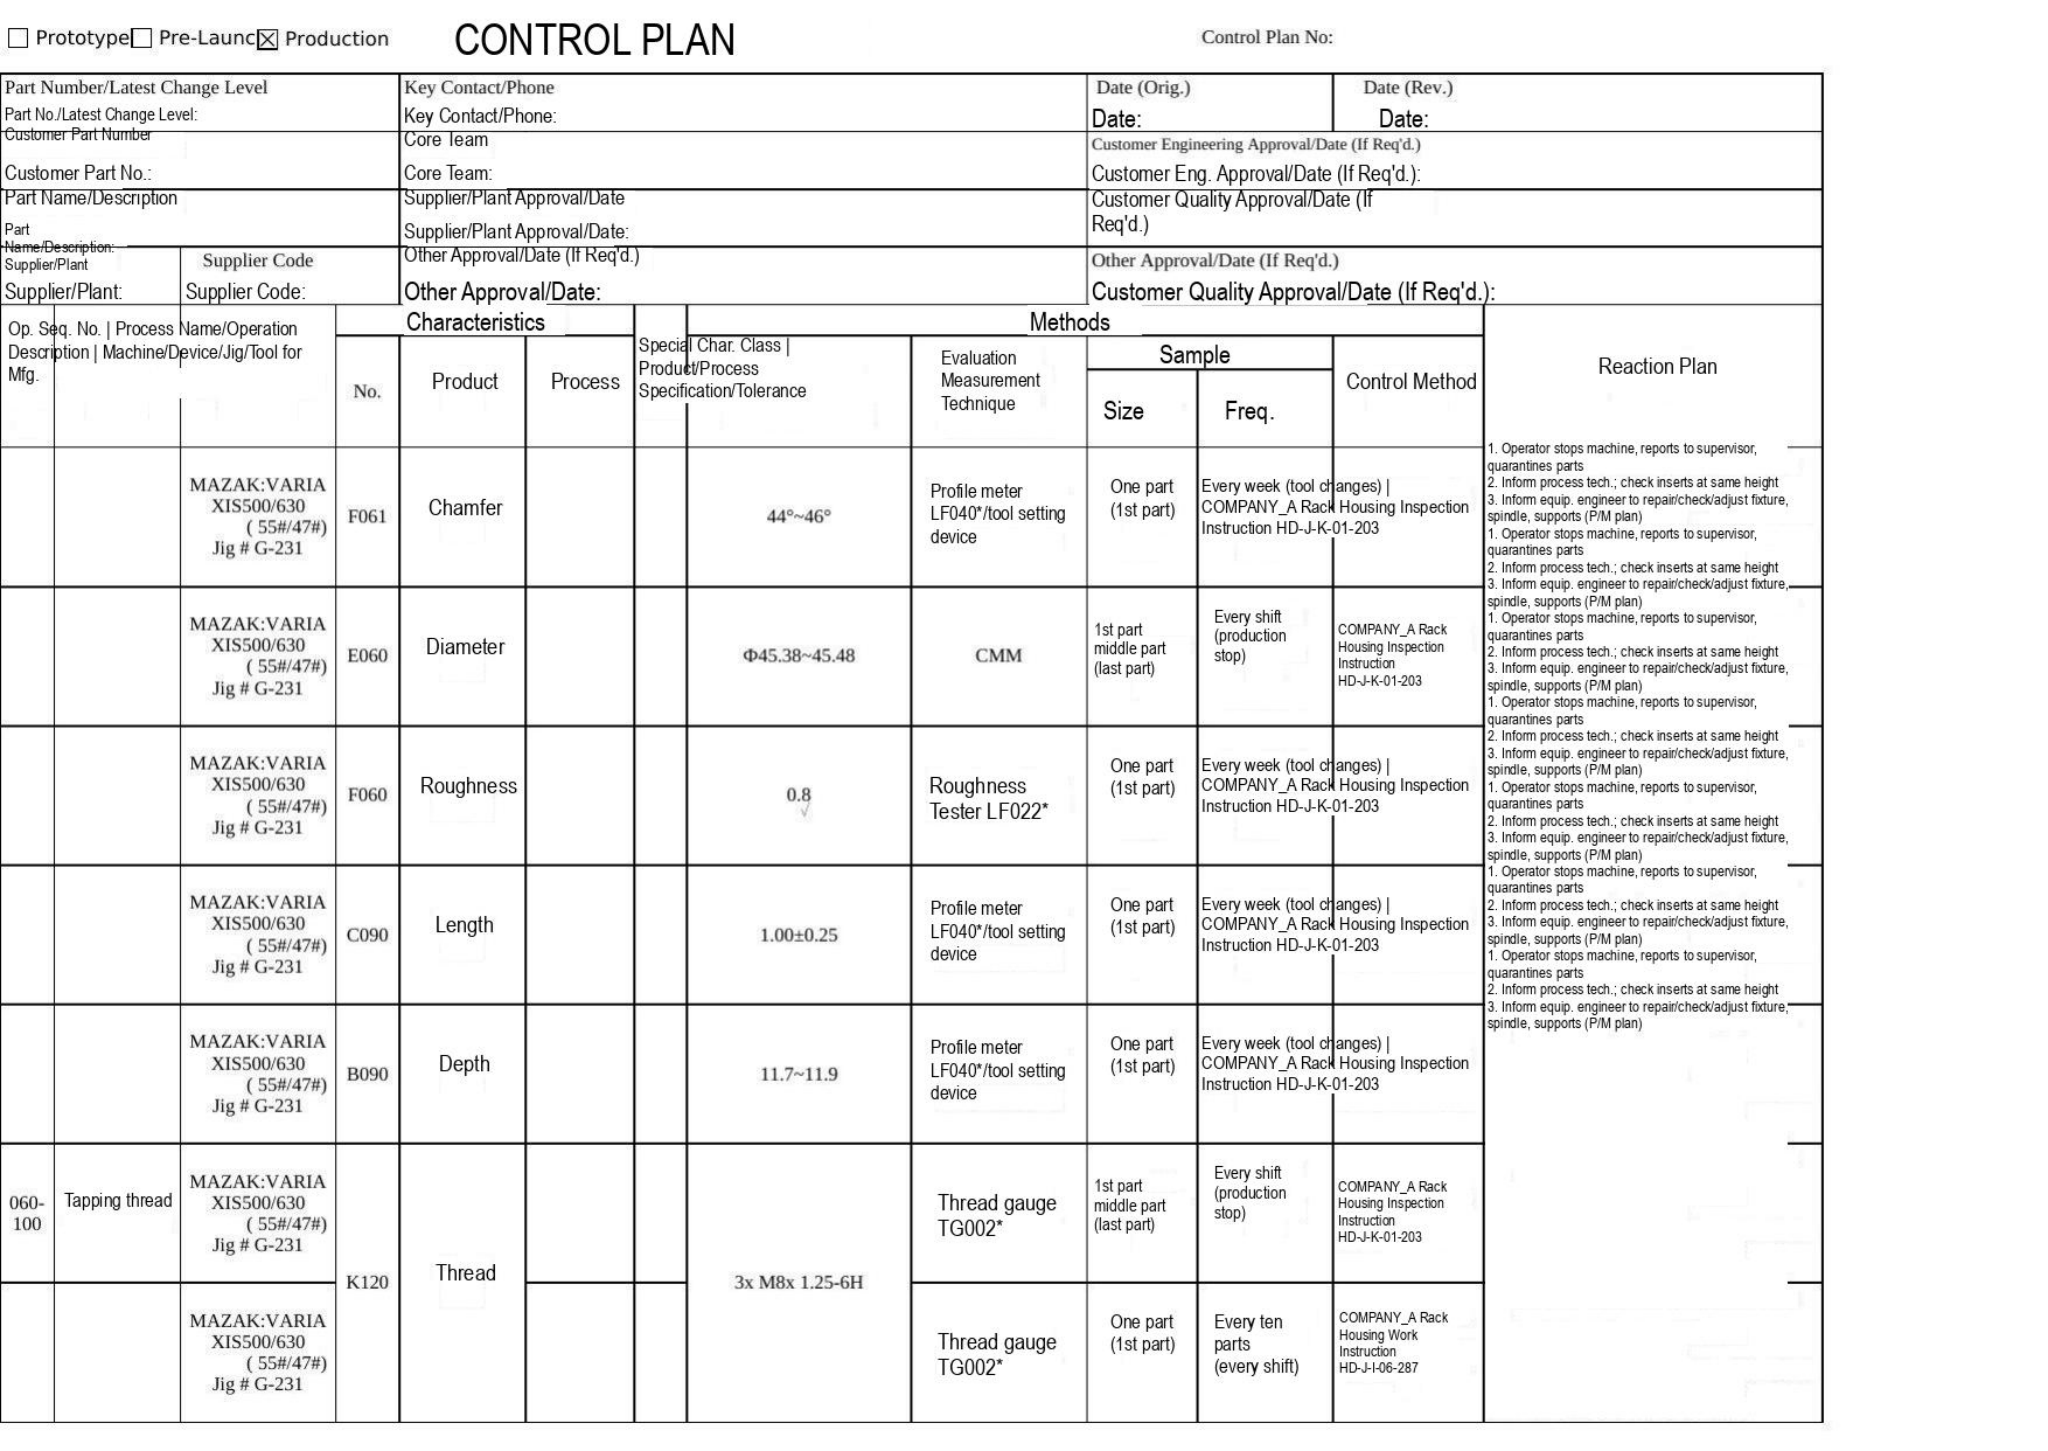☐ Prototype ☐ Pre-Launc ☒ Production

CONTROL PLAN

Control Plan No:

| Part Number/Latest Change Level<br>Part No./Latest Change Level: | | Key Contact/Phone<br>Key Contact/Phone: | Date (Orig.)<br>Date: | Date (Rev.)<br>Date: |
|---|---|---|---|---|
| Customer Part Number<br>Customer Part No.: | | Core Team<br>Core Team: | Customer Engineering Approval/Date (If Req'd.)<br>Customer Eng. Approval/Date (If Req'd.): | |
| Part Name/Description<br>Part Name/Description: | | Supplier/Plant Approval/Date<br>Supplier/Plant Approval/Date: | Customer Quality Approval/Date (If Req'd.) | |
| Supplier/Plant<br>Supplier/Plant: | Supplier Code<br>Supplier Code: | Other Approval/Date (If Req'd.)<br>Other Approval/Date: | Other Approval/Date (If Req'd.)<br>Customer Quality Approval/Date (If Req'd.): | |

| Op. Seq. No. | Process Name/Operation Description | Machine/Device/Jig/Tool for Mfg. | Characteristics<br>No. | Characteristics<br>Product | Characteristics<br>Process | Special Char. Class | Product/Process Specification/Tolerance | Methods<br>Evaluation Measurement Technique | Sample<br>Size | Sample<br>Freq. | Control Method | Reaction Plan |
|---|---|---|---|---|---|---|---|---|---|---|---|---|
| | | MAZAK:VARIA XIS500/630 ( 55#/47#) Jig # G-231 | F061 | Chamfer | | | 44°~46° | Profile meter LF040*/tool setting device | One part (1st part) | Every week (tool changes) \| | COMPANY_A Rack Housing Inspection Instruction HD-J-K-01-203 | 1. Operator stops machine, reports to supervisor, quarantines parts 2. Inform process tech.; check inserts at same height 3. Inform equip. engineer to repair/check/adjust fixture, spindle, supports (P/M plan) |
| | | MAZAK:VARIA XIS500/630 ( 55#/47#) Jig # G-231 | E060 | Diameter | | | Φ45.38~45.48 | CMM | 1st part middle part (last part) | Every shift (production stop) | COMPANY_A Rack Housing Inspection Instruction HD-J-K-01-203 | 1. Operator stops machine, reports to supervisor, quarantines parts 2. Inform process tech.; check inserts at same height 3. Inform equip. engineer to repair/check/adjust fixture, spindle, supports (P/M plan) |
| | | MAZAK:VARIA XIS500/630 ( 55#/47#) Jig # G-231 | F060 | Roughness | | | 0.8 | Roughness Tester LF022* | One part (1st part) | Every week (tool changes) \| | COMPANY_A Rack Housing Inspection Instruction HD-J-K-01-203 | 1. Operator stops machine, reports to supervisor, quarantines parts 2. Inform process tech.; check inserts at same height 3. Inform equip. engineer to repair/check/adjust fixture, spindle, supports (P/M plan) |
| | | MAZAK:VARIA XIS500/630 ( 55#/47#) Jig # G-231 | C090 | Length | | | 1.00±0.25 | Profile meter LF040*/tool setting device | One part (1st part) | Every week (tool changes) \| | COMPANY_A Rack Housing Inspection Instruction HD-J-K-01-203 | 1. Operator stops machine, reports to supervisor, quarantines parts 2. Inform process tech.; check inserts at same height 3. Inform equip. engineer to repair/check/adjust fixture, spindle, supports (P/M plan) |
| | | MAZAK:VARIA XIS500/630 ( 55#/47#) Jig # G-231 | B090 | Depth | | | 11.7~11.9 | Profile meter LF040*/tool setting device | One part (1st part) | Every week (tool changes) \| | COMPANY_A Rack Housing Inspection Instruction HD-J-K-01-203 | 1. Operator stops machine, reports to supervisor, quarantines parts 2. Inform process tech.; check inserts at same height 3. Inform equip. engineer to repair/check/adjust fixture, spindle, supports (P/M plan) |
| 060-100 | Tapping thread | MAZAK:VARIA XIS500/630 ( 55#/47#) Jig # G-231 | K120 | Thread | | | 3x M8x 1.25-6H | Thread gauge TG002* | 1st part middle part (last part) | Every shift (production stop) | COMPANY_A Rack Housing Inspection Instruction HD-J-K-01-203 | 1. Operator stops machine, reports to supervisor, quarantines parts 2. Inform process tech.; check inserts at same height 3. Inform equip. engineer to repair/check/adjust fixture, spindle, supports (P/M plan) |
| | | MAZAK:VARIA XIS500/630 ( 55#/47#) Jig # G-231 | | | | | | Thread gauge TG002* | One part (1st part) | Every ten parts (every shift) | COMPANY_A Rack Housing Work Instruction HD-J-I-06-287 | 1. Operator stops machine, reports to supervisor, quarantines parts 2. Inform process tech.; check inserts at same height 3. Inform equip. engineer to repair/check/adjust fixture, spindle, supports (P/M plan) |
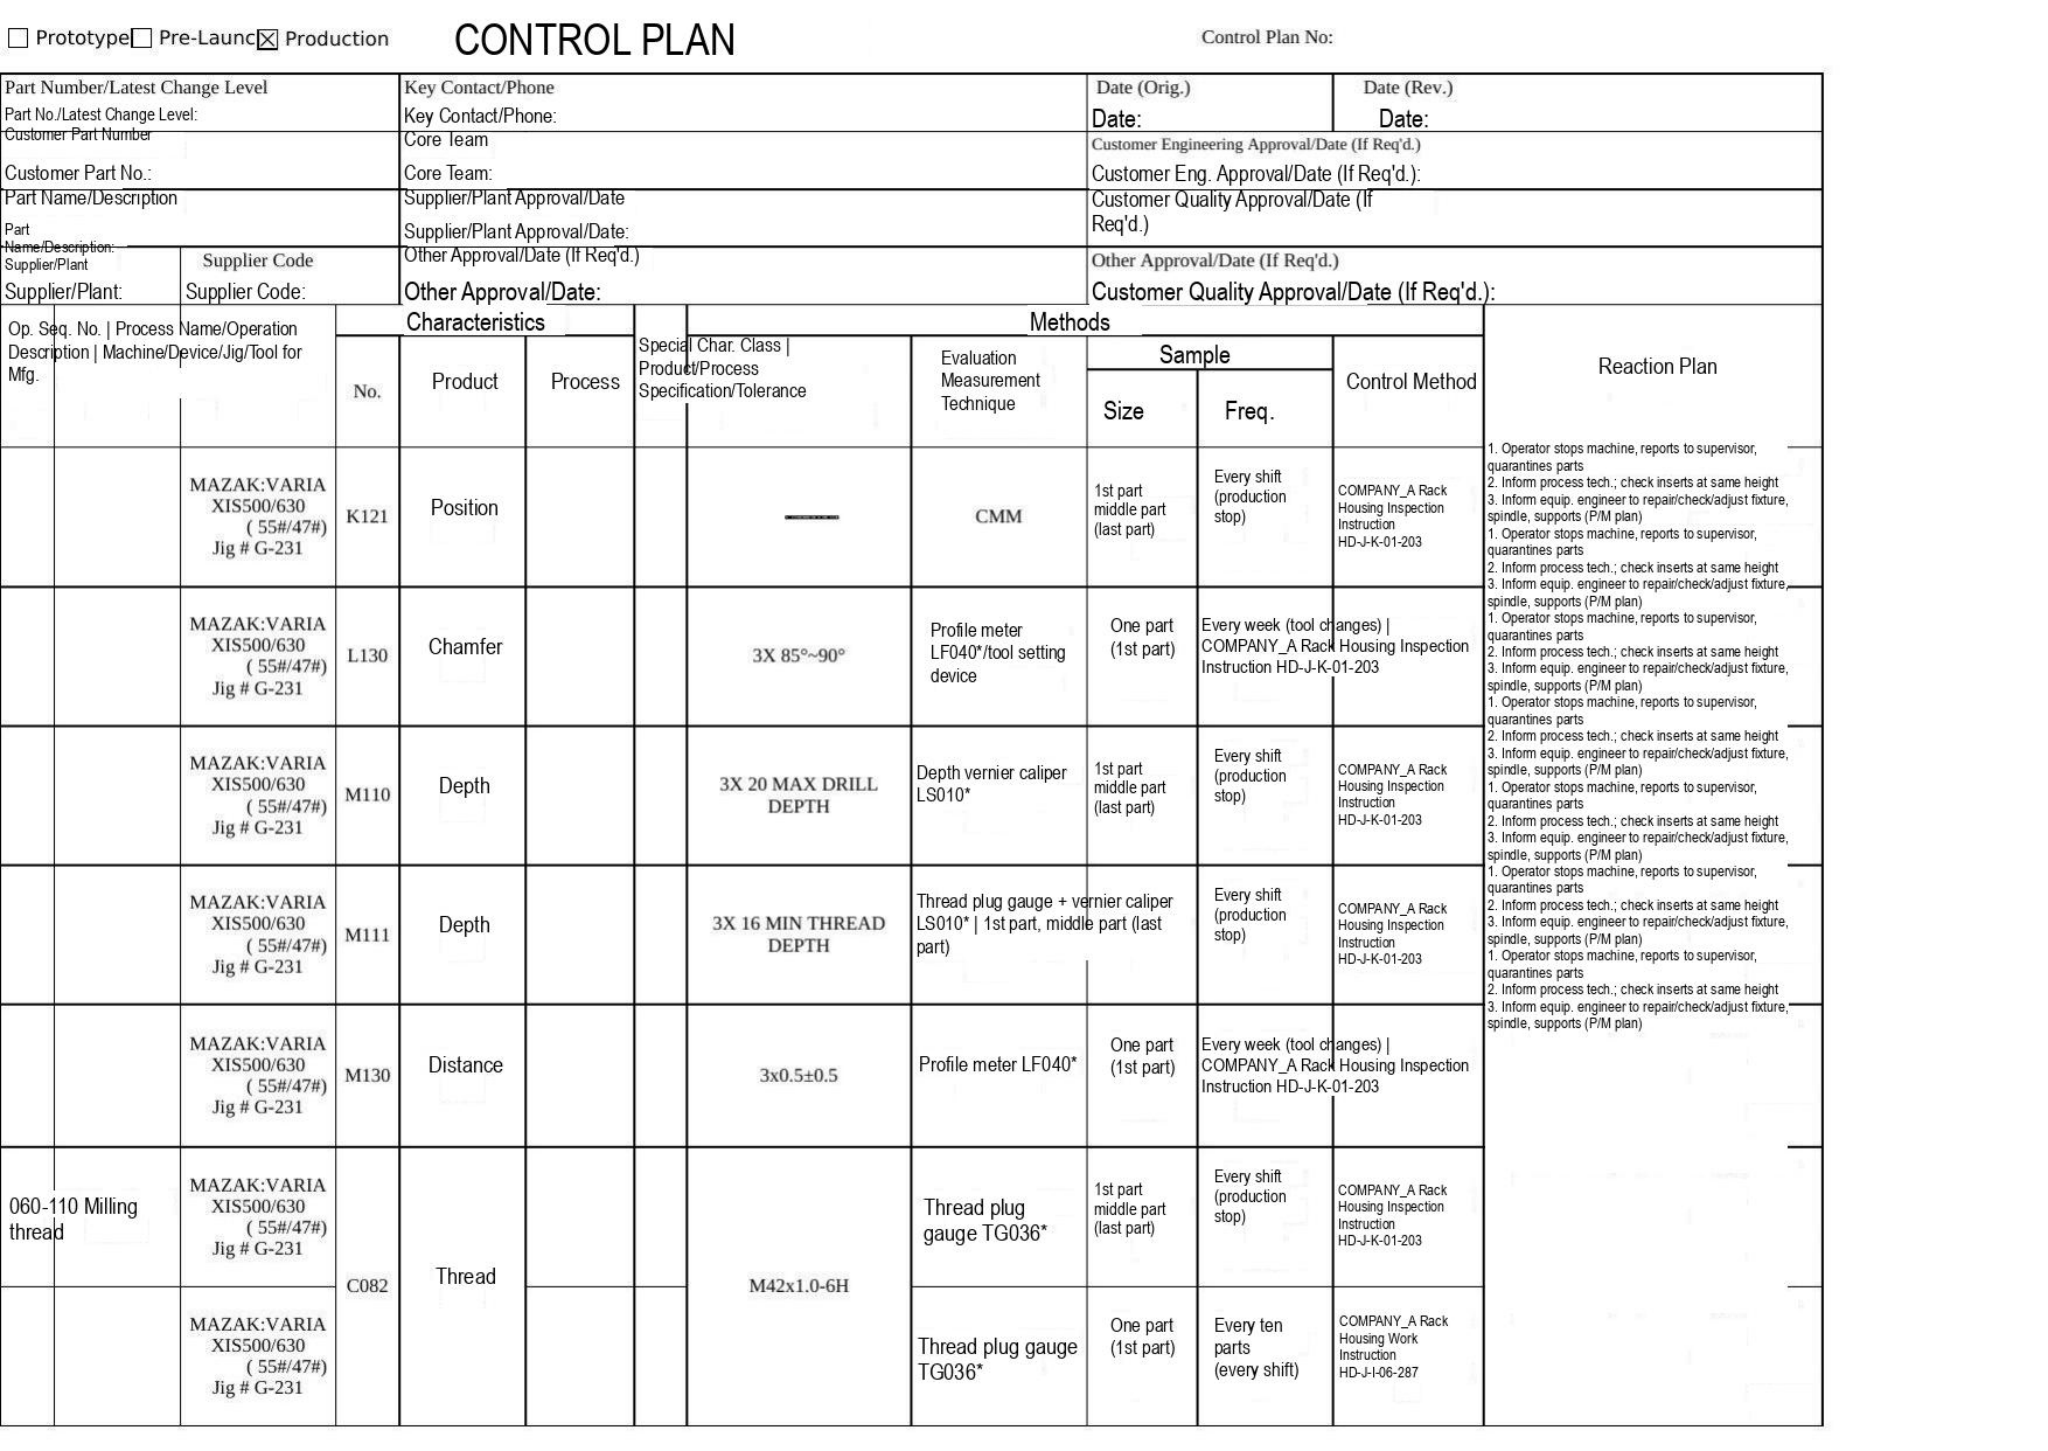☐ Prototype ☐ Pre-Launc ☒ Production

# CONTROL PLAN

Control Plan No:

| Part Number/Latest Change Level<br>Part No./Latest Change Level: | | Key Contact/Phone<br>Key Contact/Phone: | Date (Orig.)<br>Date: | Date (Rev.)<br>Date: |
|---|---|---|---|---|
| Customer Part Number<br>Customer Part No.: | | Core Team<br>Core Team: | Customer Engineering Approval/Date (If Req'd.)<br>Customer Eng. Approval/Date (If Req'd.): | |
| Part Name/Description<br>Part Name/Description: | | Supplier/Plant Approval/Date<br>Supplier/Plant Approval/Date: | Customer Quality Approval/Date (If Req'd.) | |
| Supplier/Plant<br>Supplier/Plant: | Supplier Code<br>Supplier Code: | Other Approval/Date (If Req'd.)<br>Other Approval/Date: | Other Approval/Date (If Req'd.)<br>Customer Quality Approval/Date (If Req'd.): | |

| Op. Seq. No. \| Process Name/Operation Description \| Machine/Device/Jig/Tool for Mfg. | | | Characteristics | | | | | Methods | | | | Reaction Plan |
|---|---|---|---|---|---|---|---|---|---|---|---|---|
| | | | No. | Product | Process | Special Char. Class \| Product/Process Specification/Tolerance | | Evaluation Measurement Technique | Sample Size | Sample Freq. | Control Method | |
| | | MAZAK:VARIA XIS500/630 ( 55#/47#) Jig # G-231 | K121 | Position | | | — | CMM | 1st part middle part (last part) | Every shift (production stop) | COMPANY_A Rack Housing Inspection Instruction HD-J-K-01-203 | 1. Operator stops machine, reports to supervisor, quarantines parts<br>2. Inform process tech.; check inserts at same height<br>3. Inform equip. engineer to repair/check/adjust fixture, spindle, supports (P/M plan) |
| | | MAZAK:VARIA XIS500/630 ( 55#/47#) Jig # G-231 | L130 | Chamfer | | | 3X 85°~90° | Profile meter LF040*/tool setting device | One part (1st part) | Every week (tool changes) \| COMPANY_A Rack Housing Inspection Instruction HD-J-K-01-203 | | 1. Operator stops machine, reports to supervisor, quarantines parts<br>2. Inform process tech.; check inserts at same height<br>3. Inform equip. engineer to repair/check/adjust fixture, spindle, supports (P/M plan) |
| | | MAZAK:VARIA XIS500/630 ( 55#/47#) Jig # G-231 | M110 | Depth | | | 3X 20 MAX DRILL DEPTH | Depth vernier caliper LS010* | 1st part middle part (last part) | Every shift (production stop) | COMPANY_A Rack Housing Inspection Instruction HD-J-K-01-203 | 1. Operator stops machine, reports to supervisor, quarantines parts<br>2. Inform process tech.; check inserts at same height<br>3. Inform equip. engineer to repair/check/adjust fixture, spindle, supports (P/M plan) |
| | | MAZAK:VARIA XIS500/630 ( 55#/47#) Jig # G-231 | M111 | Depth | | | 3X 16 MIN THREAD DEPTH | Thread plug gauge + vernier caliper LS010* \| 1st part, middle part (last part) | | Every shift (production stop) | COMPANY_A Rack Housing Inspection Instruction HD-J-K-01-203 | 1. Operator stops machine, reports to supervisor, quarantines parts<br>2. Inform process tech.; check inserts at same height<br>3. Inform equip. engineer to repair/check/adjust fixture, spindle, supports (P/M plan) |
| | | MAZAK:VARIA XIS500/630 ( 55#/47#) Jig # G-231 | M130 | Distance | | | 3x0.5±0.5 | Profile meter LF040* | One part (1st part) | Every week (tool changes) \| COMPANY_A Rack Housing Inspection Instruction HD-J-K-01-203 | | 1. Operator stops machine, reports to supervisor, quarantines parts<br>2. Inform process tech.; check inserts at same height<br>3. Inform equip. engineer to repair/check/adjust fixture, spindle, supports (P/M plan) |
| 060-110 Milling thread | | MAZAK:VARIA XIS500/630 ( 55#/47#) Jig # G-231 | C082 | Thread | | | M42x1.0-6H | Thread plug gauge TG036* | 1st part middle part (last part) | Every shift (production stop) | COMPANY_A Rack Housing Inspection Instruction HD-J-K-01-203 | 1. Operator stops machine, reports to supervisor, quarantines parts<br>2. Inform process tech.; check inserts at same height<br>3. Inform equip. engineer to repair/check/adjust fixture, spindle, supports (P/M plan) |
| | | MAZAK:VARIA XIS500/630 ( 55#/47#) Jig # G-231 | | | | | | Thread plug gauge TG036* | One part (1st part) | Every ten parts (every shift) | COMPANY_A Rack Housing Work Instruction HD-J-I-06-287 | |
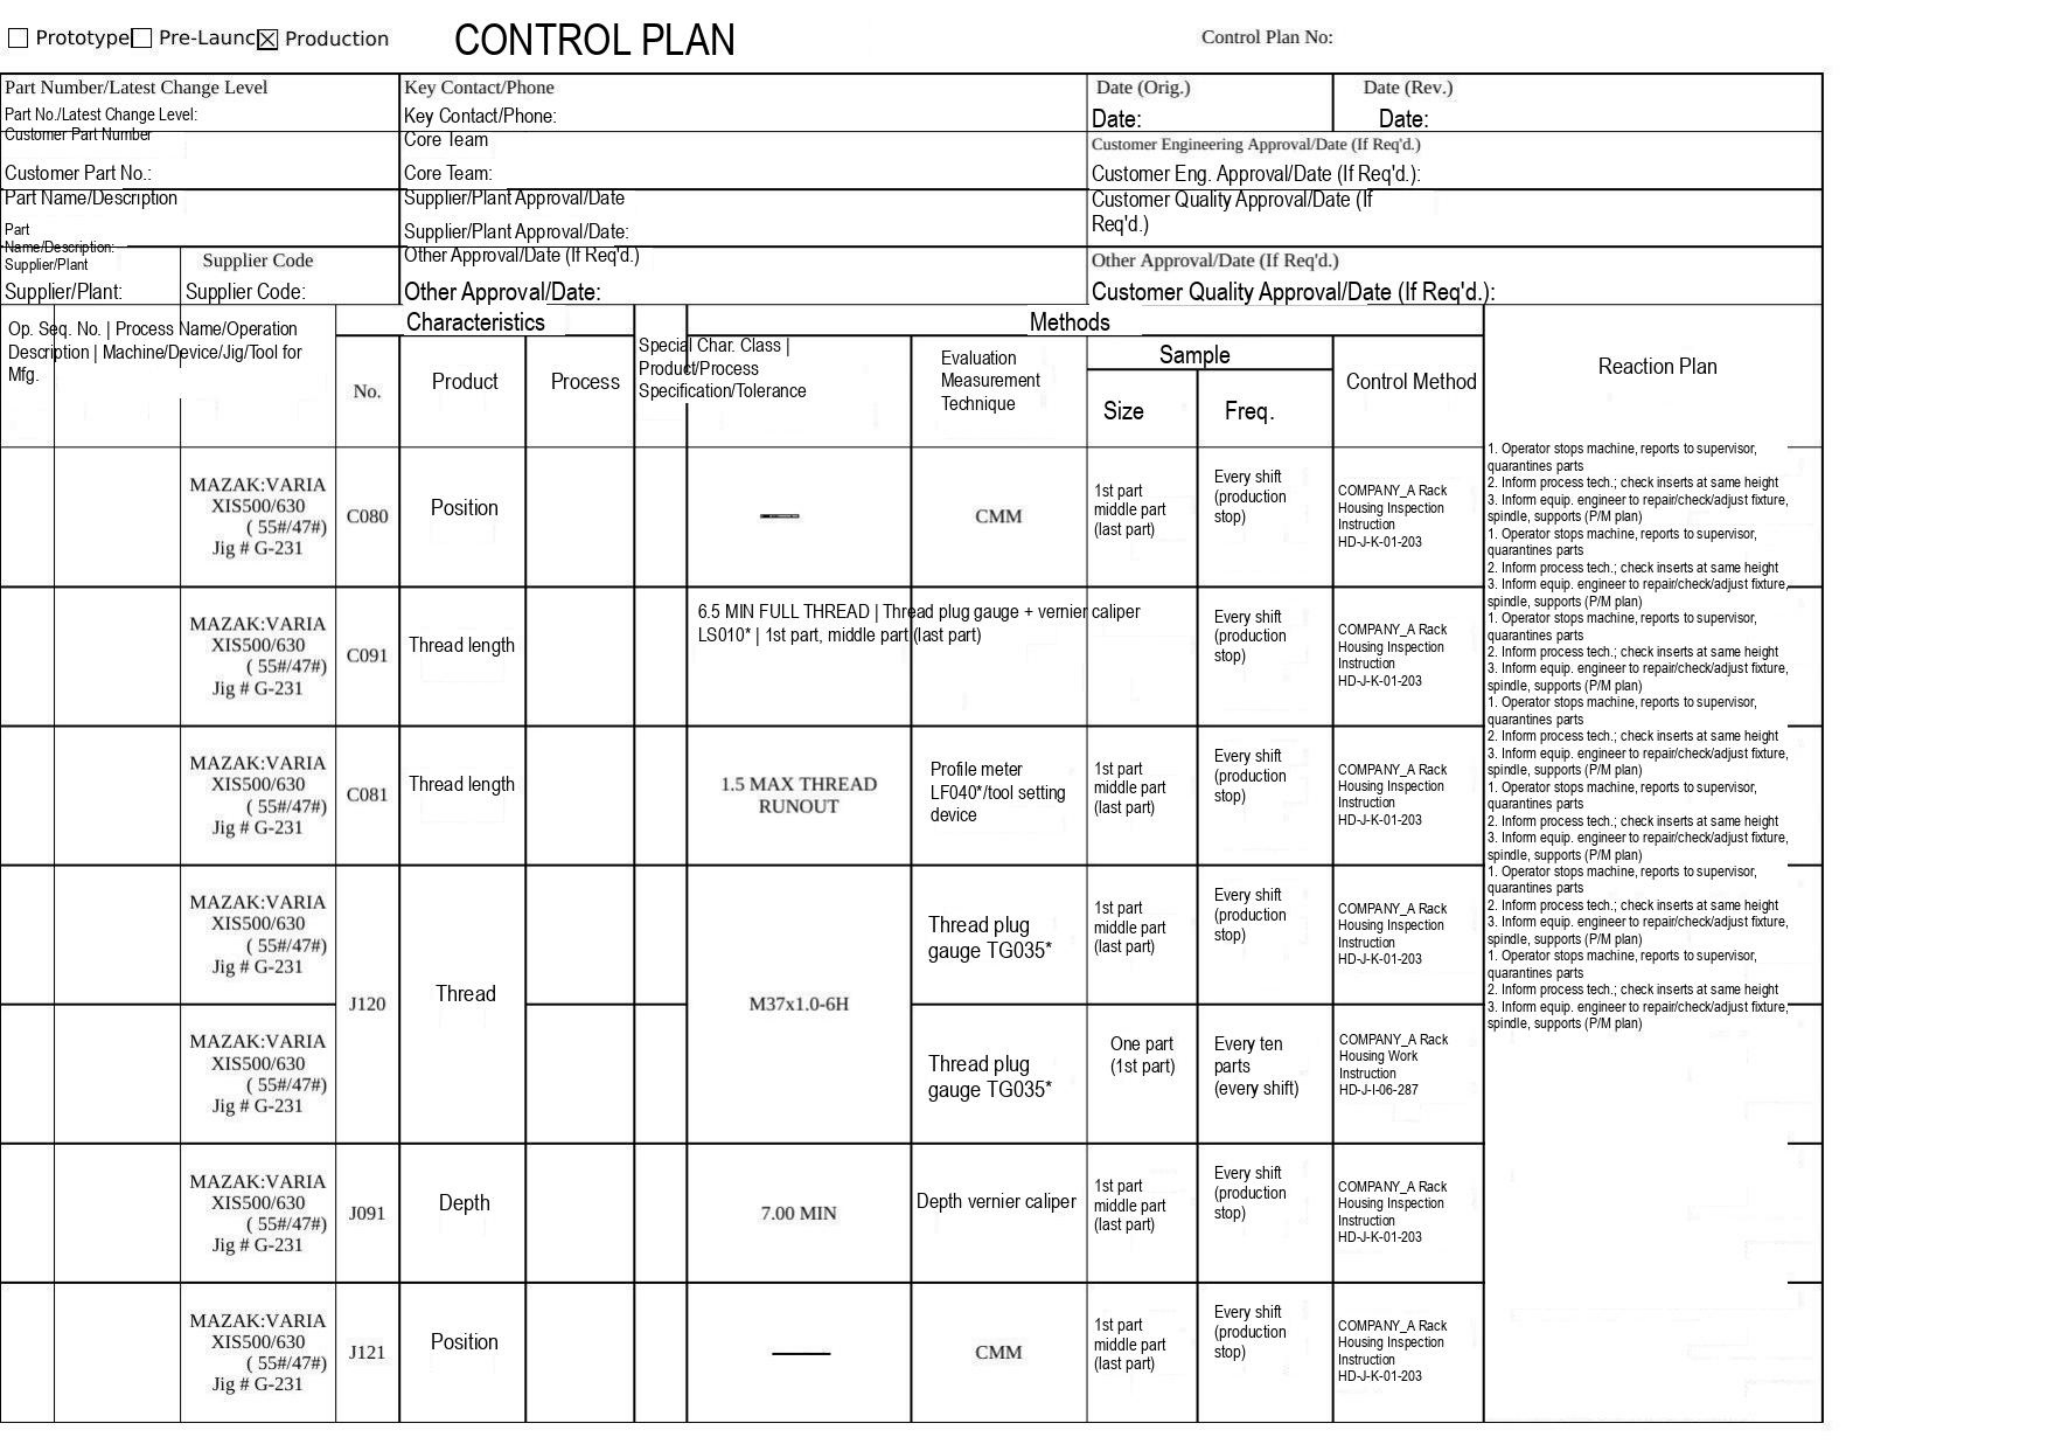☐ Prototype ☐ Pre-Launc ☒ Production

# CONTROL PLAN

Control Plan No:

| Part Number/Latest Change Level | Key Contact/Phone | Date (Orig.) | Date (Rev.) |
|---|---|---|---|
| Part No./Latest Change Level: | Key Contact/Phone: | Date: | Date: |
| Customer Part Number<br>Customer Part No.: | Core Team<br>Core Team: | Customer Engineering Approval/Date (If Req'd.)<br>Customer Eng. Approval/Date (If Req'd.): | |
| Part Name/Description<br>Part Name/Description: | Supplier/Plant Approval/Date<br>Supplier/Plant Approval/Date: | Customer Quality Approval/Date (If Req'd.) | |
| Supplier/Plant<br>Supplier/Plant: Supplier Code<br>Supplier Code: | Other Approval/Date (If Req'd.)<br>Other Approval/Date: | Other Approval/Date (If Req'd.)<br>Customer Quality Approval/Date (If Req'd.): | |

| Op. Seq. No. | Process Name/Operation Description | Machine/Device/Jig/Tool for Mfg. | Characteristics No. | Characteristics Product | Characteristics Process | Special Char. Class | Product/Process Specification/Tolerance | Methods Evaluation Measurement Technique | Methods Sample Size | Methods Sample Freq. | Methods Control Method | Reaction Plan |
|---|---|---|---|---|---|---|---|---|---|---|---|---|
| | | MAZAK:VARIA XIS500/630 ( 55#/47#) Jig # G-231 | C080 | Position | | | — | CMM | 1st part middle part (last part) | Every shift (production stop) | COMPANY_A Rack Housing Inspection Instruction HD-J-K-01-203 | 1. Operator stops machine, reports to supervisor, quarantines parts 2. Inform process tech.; check inserts at same height 3. Inform equip. engineer to repair/check/adjust fixture, spindle, supports (P/M plan) |
| | | MAZAK:VARIA XIS500/630 ( 55#/47#) Jig # G-231 | C091 | Thread length | | | 6.5 MIN FULL THREAD | Thread plug gauge + vernier caliper LS010* | 1st part, middle part (last part) | Every shift (production stop) | COMPANY_A Rack Housing Inspection Instruction HD-J-K-01-203 | 1. Operator stops machine, reports to supervisor, quarantines parts 2. Inform process tech.; check inserts at same height 3. Inform equip. engineer to repair/check/adjust fixture, spindle, supports (P/M plan) |
| | | MAZAK:VARIA XIS500/630 ( 55#/47#) Jig # G-231 | C081 | Thread length | | | 1.5 MAX THREAD RUNOUT | Profile meter LF040*/tool setting device | 1st part middle part (last part) | Every shift (production stop) | COMPANY_A Rack Housing Inspection Instruction HD-J-K-01-203 | 1. Operator stops machine, reports to supervisor, quarantines parts 2. Inform process tech.; check inserts at same height 3. Inform equip. engineer to repair/check/adjust fixture, spindle, supports (P/M plan) |
| | | MAZAK:VARIA XIS500/630 ( 55#/47#) Jig # G-231 | J120 | Thread | | | M37x1.0-6H | Thread plug gauge TG035* | 1st part middle part (last part) | Every shift (production stop) | COMPANY_A Rack Housing Inspection Instruction HD-J-K-01-203 | 1. Operator stops machine, reports to supervisor, quarantines parts 2. Inform process tech.; check inserts at same height 3. Inform equip. engineer to repair/check/adjust fixture, spindle, supports (P/M plan) |
| | | MAZAK:VARIA XIS500/630 ( 55#/47#) Jig # G-231 | | | | | | Thread plug gauge TG035* | One part (1st part) | Every ten parts (every shift) | COMPANY_A Rack Housing Work Instruction HD-J-I-06-287 | 1. Operator stops machine, reports to supervisor, quarantines parts 2. Inform process tech.; check inserts at same height 3. Inform equip. engineer to repair/check/adjust fixture, spindle, supports (P/M plan) |
| | | MAZAK:VARIA XIS500/630 ( 55#/47#) Jig # G-231 | J091 | Depth | | | 7.00 MIN | Depth vernier caliper | 1st part middle part (last part) | Every shift (production stop) | COMPANY_A Rack Housing Inspection Instruction HD-J-K-01-203 | 1. Operator stops machine, reports to supervisor, quarantines parts 2. Inform process tech.; check inserts at same height 3. Inform equip. engineer to repair/check/adjust fixture, spindle, supports (P/M plan) |
| | | MAZAK:VARIA XIS500/630 ( 55#/47#) Jig # G-231 | J121 | Position | | | — | CMM | 1st part middle part (last part) | Every shift (production stop) | COMPANY_A Rack Housing Inspection Instruction HD-J-K-01-203 | 1. Operator stops machine, reports to supervisor, quarantines parts 2. Inform process tech.; check inserts at same height 3. Inform equip. engineer to repair/check/adjust fixture, spindle, supports (P/M plan) |
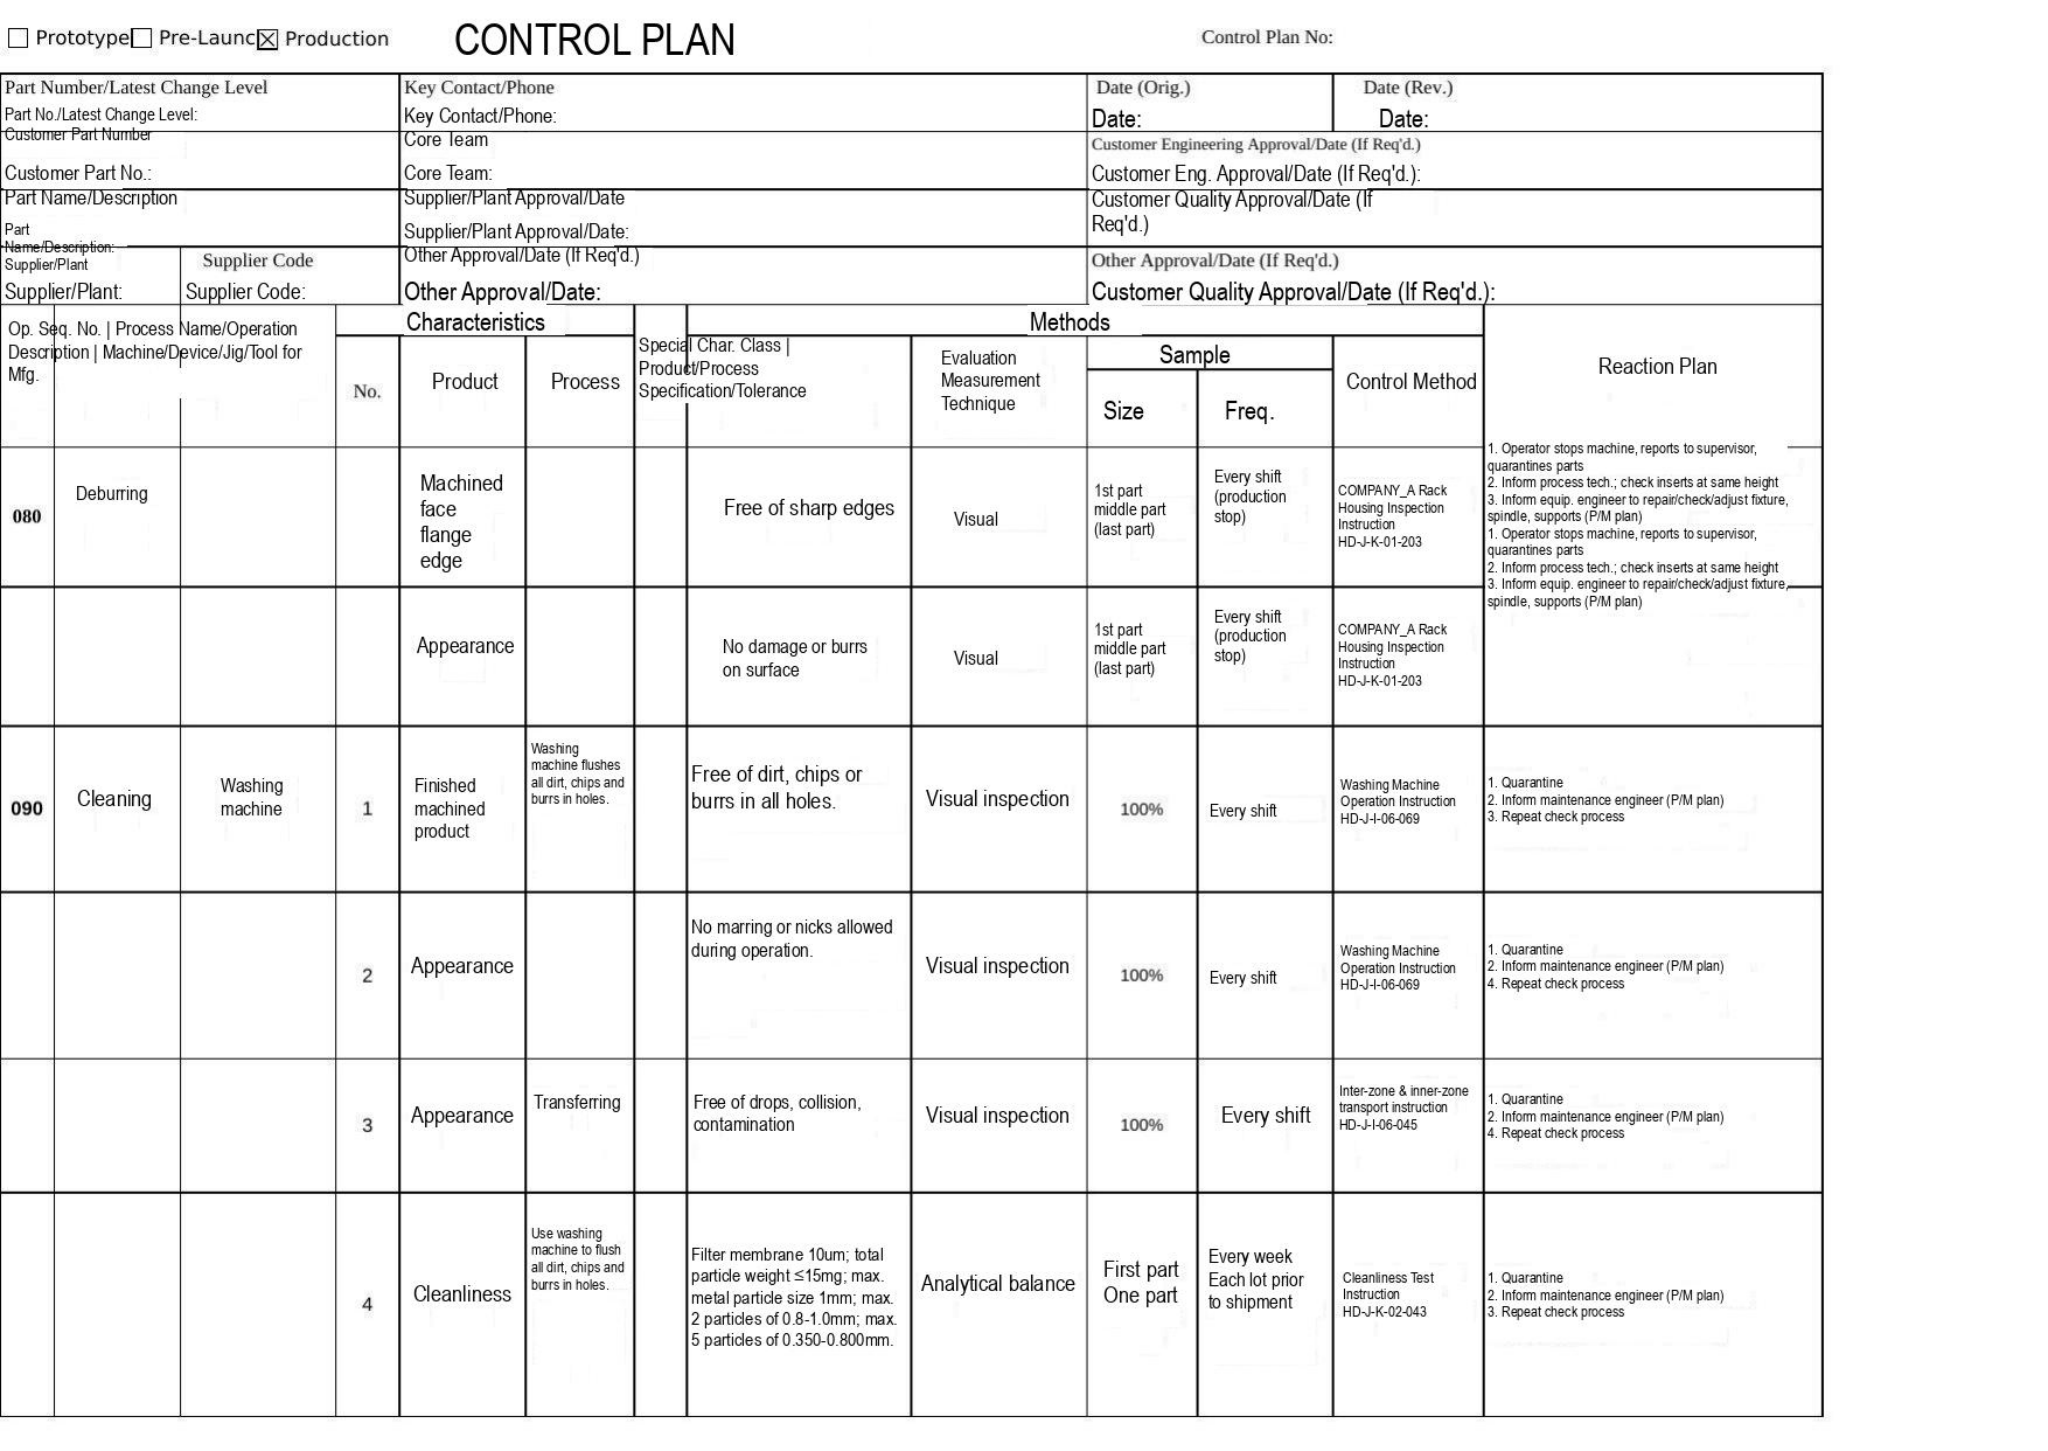☐ Prototype ☐ Pre-Launc ☒ Production

CONTROL PLAN

Control Plan No:

| Part Number/Latest Change Level<br>Part No./Latest Change Level: | Key Contact/Phone<br>Key Contact/Phone: | Date (Orig.)<br>Date: | Date (Rev.)<br>Date: |
|---|---|---|---|
| Customer Part Number<br>Customer Part No.: | Core Team<br>Core Team: | Customer Engineering Approval/Date (If Req'd.)<br>Customer Eng. Approval/Date (If Req'd.): | |
| Part Name/Description<br>Part Name/Description: | Supplier/Plant Approval/Date<br>Supplier/Plant Approval/Date: | Customer Quality Approval/Date (If Req'd.) | |
| Supplier/Plant<br>Supplier/Plant: / Supplier Code<br>Supplier Code: | Other Approval/Date (If Req'd.)<br>Other Approval/Date: | Other Approval/Date (If Req'd.)<br>Customer Quality Approval/Date (If Req'd.): | |

| Op. Seq. No. | Process Name/Operation Description | Machine/Device/Jig/Tool for Mfg. | Characteristics No. | Characteristics Product | Characteristics Process | Special Char. Class | Methods Product/Process Specification/Tolerance | Methods Evaluation Measurement Technique | Methods Sample Size | Methods Sample Freq. | Methods Control Method | Reaction Plan |
|---|---|---|---|---|---|---|---|---|---|---|---|---|
| 080 | Deburring | | | Machined face flange edge | | | Free of sharp edges | Visual | 1st part middle part (last part) | Every shift (production stop) | COMPANY_A Rack Housing Inspection Instruction HD-J-K-01-203 | 1. Operator stops machine, reports to supervisor, quarantines parts<br>2. Inform process tech.; check inserts at same height<br>3. Inform equip. engineer to repair/check/adjust fixture, spindle, supports (P/M plan)<br>1. Operator stops machine, reports to supervisor, quarantines parts<br>2. Inform process tech.; check inserts at same height<br>3. Inform equip. engineer to repair/check/adjust fixture, spindle, supports (P/M plan) |
| | | | | Appearance | | | No damage or burrs on surface | Visual | 1st part middle part (last part) | Every shift (production stop) | COMPANY_A Rack Housing Inspection Instruction HD-J-K-01-203 | |
| 090 | Cleaning | Washing machine | 1 | Finished machined product | Washing machine flushes all dirt, chips and burrs in holes. | | Free of dirt, chips or burrs in all holes. | Visual inspection | 100% | Every shift | Washing Machine Operation Instruction HD-J-I-06-069 | 1. Quarantine<br>2. Inform maintenance engineer (P/M plan)<br>3. Repeat check process |
| | | | 2 | Appearance | | | No marring or nicks allowed during operation. | Visual inspection | 100% | Every shift | Washing Machine Operation Instruction HD-J-I-06-069 | 1. Quarantine<br>2. Inform maintenance engineer (P/M plan)<br>4. Repeat check process |
| | | | 3 | Appearance | Transferring | | Free of drops, collision, contamination | Visual inspection | 100% | Every shift | Inter-zone & inner-zone transport instruction HD-J-I-06-045 | 1. Quarantine<br>2. Inform maintenance engineer (P/M plan)<br>4. Repeat check process |
| | | | 4 | Cleanliness | Use washing machine to flush all dirt, chips and burrs in holes. | | Filter membrane 10um; total particle weight ≤15mg; max. metal particle size 1mm; max. 2 particles of 0.8-1.0mm; max. 5 particles of 0.350-0.800mm. | Analytical balance | First part One part | Every week Each lot prior to shipment | Cleanliness Test Instruction HD-J-K-02-043 | 1. Quarantine<br>2. Inform maintenance engineer (P/M plan)<br>3. Repeat check process |
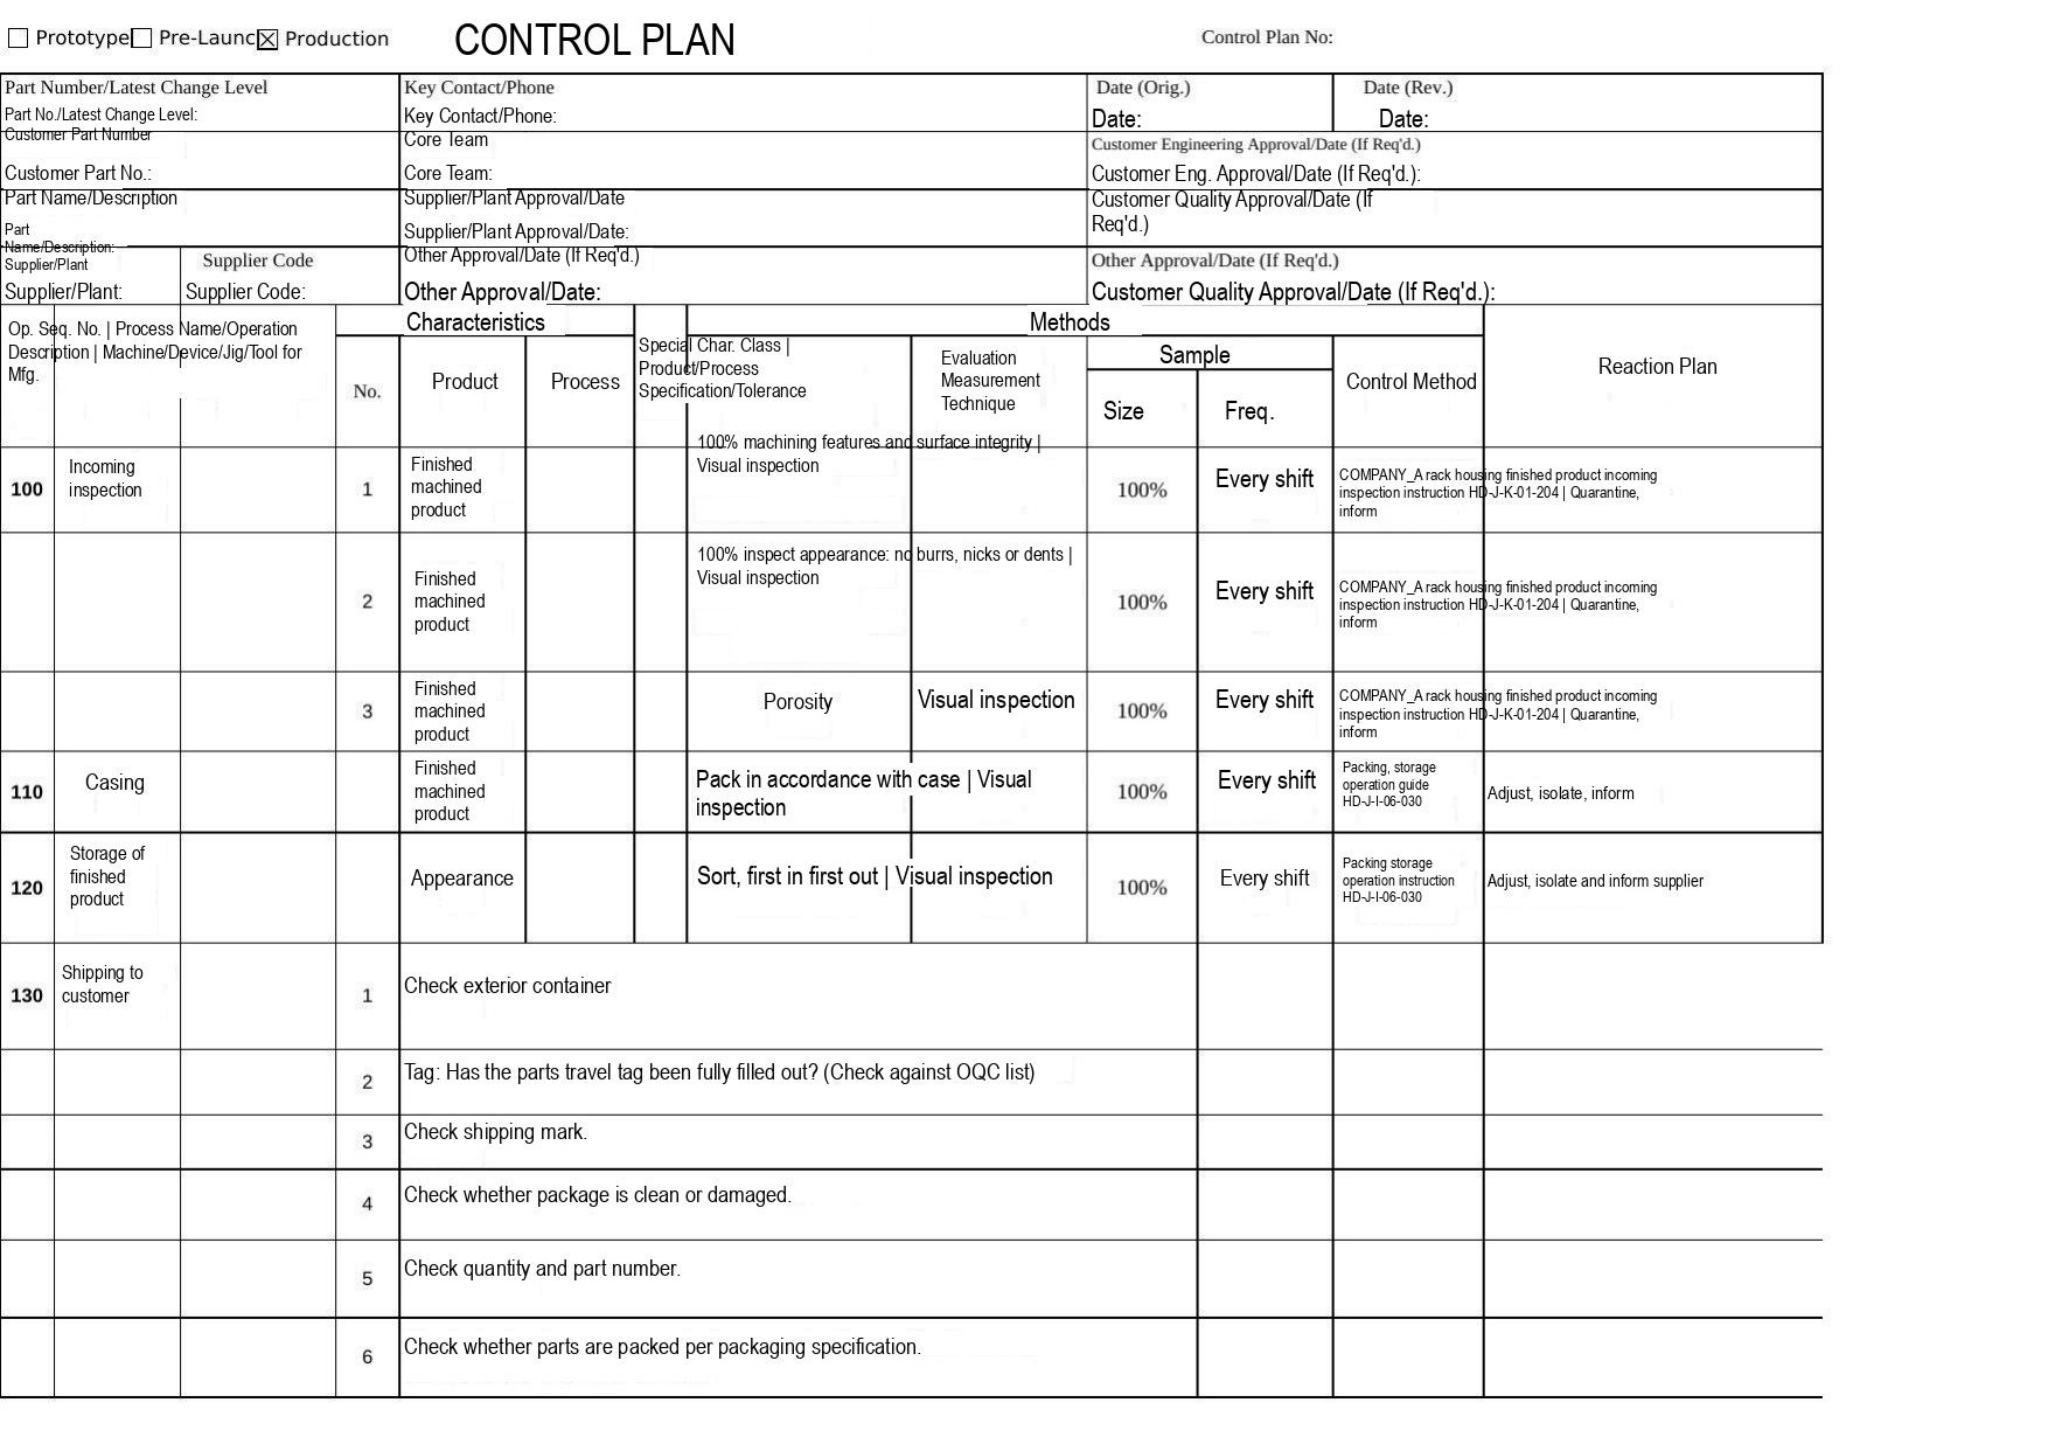☐ Prototype ☐ Pre-Launc ☒ Production CONTROL PLAN Control Plan No:

| Part Number/Latest Change Level | Key Contact/Phone | Date (Orig.) | Date (Rev.) |
|---|---|---|---|
| Part No./Latest Change Level: | Key Contact/Phone: | Date: | Date: |
| Customer Part Number | Core Team | Customer Engineering Approval/Date (If Req'd.) | |
| Customer Part No.: | Core Team: | Customer Eng. Approval/Date (If Req'd.): | |
| Part Name/Description | Supplier/Plant Approval/Date | Customer Quality Approval/Date (If Req'd.) | |
| Part Name/Description: | Supplier/Plant Approval/Date: | | |
| Supplier/Plant / Supplier Code | Other Approval/Date (If Req'd.) | Other Approval/Date (If Req'd.) | |
| Supplier/Plant: / Supplier Code: | Other Approval/Date: | Customer Quality Approval/Date (If Req'd.): | |

| Op. Seq. No. | Process Name/Operation Description | Machine/Device/Jig/Tool for Mfg. | Characteristics No. | Characteristics Product | Characteristics Process | Special Char. Class | Methods Product/Process Specification/Tolerance | Methods Evaluation Measurement Technique | Sample Size | Sample Freq. | Control Method | Reaction Plan |
|---|---|---|---|---|---|---|---|---|---|---|---|---|
| 100 | Incoming inspection | | 1 | Finished machined product | | | 100% machining features and surface integrity \| Visual inspection | | 100% | Every shift | COMPANY_A rack housing finished product incoming inspection instruction HD-J-K-01-204 \| Quarantine, inform | |
| | | | 2 | Finished machined product | | | 100% inspect appearance: no burrs, nicks or dents \| Visual inspection | | 100% | Every shift | COMPANY_A rack housing finished product incoming inspection instruction HD-J-K-01-204 \| Quarantine, inform | |
| | | | 3 | Finished machined product | | | Porosity | Visual inspection | 100% | Every shift | COMPANY_A rack housing finished product incoming inspection instruction HD-J-K-01-204 \| Quarantine, inform | |
| 110 | Casing | | | Finished machined product | | | Pack in accordance with case \| Visual inspection | | 100% | Every shift | Packing, storage operation guide HD-J-I-06-030 | Adjust, isolate, inform |
| 120 | Storage of finished product | | | Appearance | | | Sort, first in first out \| Visual inspection | | 100% | Every shift | Packing storage operation instruction HD-J-I-06-030 | Adjust, isolate and inform supplier |
| 130 | Shipping to customer | | 1 | Check exterior container | | | | | | | | |
| | | | 2 | Tag: Has the parts travel tag been fully filled out? (Check against OQC list) | | | | | | | | |
| | | | 3 | Check shipping mark. | | | | | | | | |
| | | | 4 | Check whether package is clean or damaged. | | | | | | | | |
| | | | 5 | Check quantity and part number. | | | | | | | | |
| | | | 6 | Check whether parts are packed per packaging specification. | | | | | | | | |